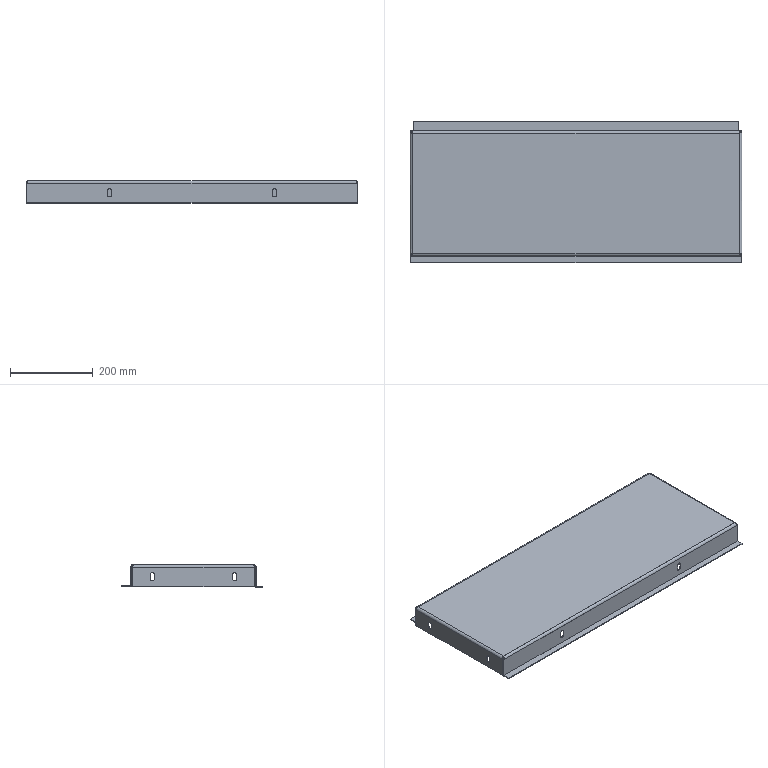Part | STEP file | SYL_0392D6J1SYL0380DJ100-373455 | 1 solid | 92 faces | box 804 x 343 x 55 mm | volume 764236 mm3 | plane 54 | cylinder 30 | spline 8 | commonest cylinder face diameters 10 x20 8 x4 12 x4 4 x2